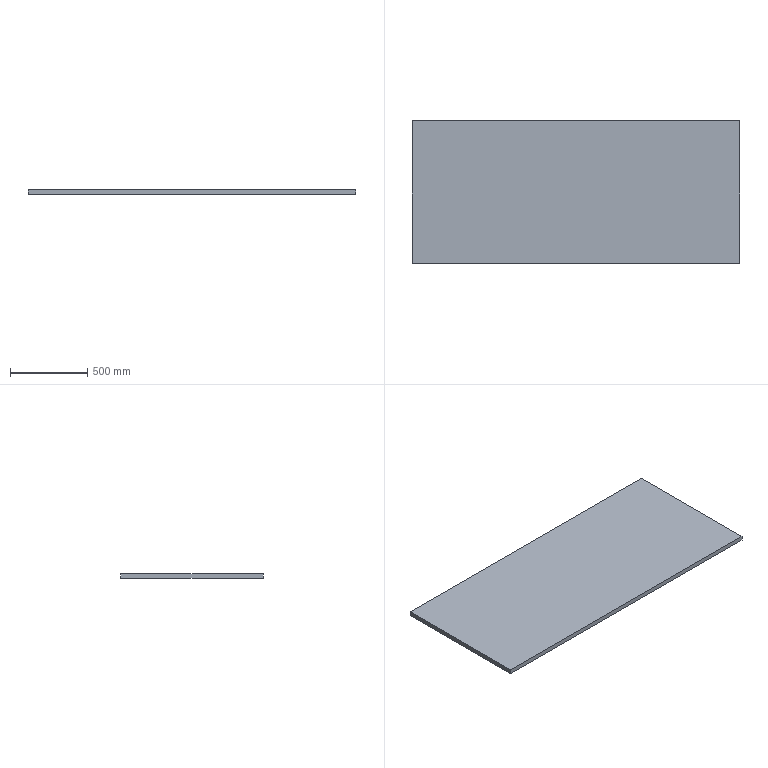Part | SolidWorks | features Extrusion 1 | 1 solid | 6 faces | box 2118 x 922 x 30 mm | volume 58583880 mm3 | plane 6
STEP:
#1=CARTESIAN_POINT('',(0.,922.,0.));
#2=VERTEX_POINT('',#1);
#3=CARTESIAN_POINT('',(0.,0.,0.));
#4=VERTEX_POINT('',#3);
#5=CARTESIAN_POINT('',(0.,0.,0.));
#6=DIRECTION('',(0.,-1.,0.));
#7=VECTOR('',#6,1000.);
#8=LINE('',#5,#7);
#9=EDGE_CURVE('',#2,#4,#8,.T.);
#10=ORIENTED_EDGE('',*,*,#9,.T.);
#11=CARTESIAN_POINT('',(0.,0.,30.));
#12=VERTEX_POINT('',#11);
#13=CARTESIAN_POINT('',(0.,0.,30.));
#14=DIRECTION('',(0.,0.,-1.));
#15=VECTOR('',#14,1000.);
#16=LINE('',#13,#15);
#17=EDGE_CURVE('',#12,#4,#16,.T.);
#18=ORIENTED_EDGE('',*,*,#17,.F.);
#19=CARTESIAN_POINT('',(0.,922.,30.));
#20=VERTEX_POINT('',#19);
#21=CARTESIAN_POINT('',(0.,0.,30.));
#22=DIRECTION('',(0.,-1.,0.));
#23=VECTOR('',#22,1000.);
#24=LINE('',#21,#23);
#25=EDGE_CURVE('',#20,#12,#24,.T.);
#26=ORIENTED_EDGE('',*,*,#25,.F.);
#27=CARTESIAN_POINT('',(0.,922.,30.));
#28=DIRECTION('',(0.,0.,-1.));
#29=VECTOR('',#28,1000.);
#30=LINE('',#27,#29);
#31=EDGE_CURVE('',#20,#2,#30,.T.);
#32=ORIENTED_EDGE('',*,*,#31,.T.);
#33=EDGE_LOOP('',(#10,#18,#26,#32));
#34=FACE_OUTER_BOUND('',#33,.T.);
#35=CARTESIAN_POINT('',(0.,0.,30.));
#36=DIRECTION('',(1.,0.,0.));
#37=DIRECTION('',(0.,0.,-1.));
#38=AXIS2_PLACEMENT_3D('',#35,#36,#37);
#39=PLANE('',#38);
#40=ADVANCED_FACE('',(#34),#39,.F.);
#41=CARTESIAN_POINT('',(2118.,0.,0.));
#42=VERTEX_POINT('',#41);
#43=CARTESIAN_POINT('',(0.,0.,0.));
#44=DIRECTION('',(1.,0.,0.));
#45=VECTOR('',#44,1000.);
#46=LINE('',#43,#45);
#47=EDGE_CURVE('',#4,#42,#46,.T.);
#48=ORIENTED_EDGE('',*,*,#47,.T.);
#49=CARTESIAN_POINT('',(2118.,0.,30.));
#50=VERTEX_POINT('',#49);
#51=CARTESIAN_POINT('',(2118.,0.,30.));
#52=DIRECTION('',(0.,0.,-1.));
#53=VECTOR('',#52,1000.);
#54=LINE('',#51,#53);
#55=EDGE_CURVE('',#50,#42,#54,.T.);
#56=ORIENTED_EDGE('',*,*,#55,.F.);
#57=CARTESIAN_POINT('',(0.,0.,30.));
#58=DIRECTION('',(1.,0.,0.));
#59=VECTOR('',#58,1000.);
#60=LINE('',#57,#59);
#61=EDGE_CURVE('',#12,#50,#60,.T.);
#62=ORIENTED_EDGE('',*,*,#61,.F.);
#63=ORIENTED_EDGE('',*,*,#17,.T.);
#64=EDGE_LOOP('',(#48,#56,#62,#63));
#65=FACE_OUTER_BOUND('',#64,.T.);
#66=CARTESIAN_POINT('',(0.,0.,30.));
#67=DIRECTION('',(0.,1.,0.));
#68=DIRECTION('',(0.,0.,1.));
#69=AXIS2_PLACEMENT_3D('',#66,#67,#68);
#70=PLANE('',#69);
#71=ADVANCED_FACE('',(#65),#70,.F.);
#72=CARTESIAN_POINT('',(2118.,922.,0.));
#73=VERTEX_POINT('',#72);
#74=CARTESIAN_POINT('',(2118.,0.,0.));
#75=DIRECTION('',(0.,1.,0.));
#76=VECTOR('',#75,1000.);
#77=LINE('',#74,#76);
#78=EDGE_CURVE('',#42,#73,#77,.T.);
#79=ORIENTED_EDGE('',*,*,#78,.T.);
#80=CARTESIAN_POINT('',(2118.,922.,30.));
#81=VERTEX_POINT('',#80);
#82=CARTESIAN_POINT('',(2118.,922.,30.));
#83=DIRECTION('',(0.,0.,-1.));
#84=VECTOR('',#83,1000.);
#85=LINE('',#82,#84);
#86=EDGE_CURVE('',#81,#73,#85,.T.);
#87=ORIENTED_EDGE('',*,*,#86,.F.);
#88=CARTESIAN_POINT('',(2118.,0.,30.));
#89=DIRECTION('',(0.,1.,0.));
#90=VECTOR('',#89,1000.);
#91=LINE('',#88,#90);
#92=EDGE_CURVE('',#50,#81,#91,.T.);
#93=ORIENTED_EDGE('',*,*,#92,.F.);
#94=ORIENTED_EDGE('',*,*,#55,.T.);
#95=EDGE_LOOP('',(#79,#87,#93,#94));
#96=FACE_OUTER_BOUND('',#95,.T.);
#97=CARTESIAN_POINT('',(2118.,0.,30.));
#98=DIRECTION('',(-1.,0.,0.));
#99=DIRECTION('',(0.,0.,1.));
#100=AXIS2_PLACEMENT_3D('',#97,#98,#99);
#101=PLANE('',#100);
#102=ADVANCED_FACE('',(#96),#101,.F.);
#103=CARTESIAN_POINT('',(0.,922.,0.));
#104=DIRECTION('',(-1.,0.,0.));
#105=VECTOR('',#104,1000.);
#106=LINE('',#103,#105);
#107=EDGE_CURVE('',#73,#2,#106,.T.);
#108=ORIENTED_EDGE('',*,*,#107,.T.);
#109=ORIENTED_EDGE('',*,*,#31,.F.);
#110=CARTESIAN_POINT('',(0.,922.,30.));
#111=DIRECTION('',(-1.,0.,0.));
#112=VECTOR('',#111,1000.);
#113=LINE('',#110,#112);
#114=EDGE_CURVE('',#81,#20,#113,.T.);
#115=ORIENTED_EDGE('',*,*,#114,.F.);
#116=ORIENTED_EDGE('',*,*,#86,.T.);
#117=EDGE_LOOP('',(#108,#109,#115,#116));
#118=FACE_OUTER_BOUND('',#117,.T.);
#119=CARTESIAN_POINT('',(0.,922.,30.));
#120=DIRECTION('',(0.,-1.,0.));
#121=DIRECTION('',(0.,0.,-1.));
#122=AXIS2_PLACEMENT_3D('',#119,#120,#121);
#123=PLANE('',#122);
#124=ADVANCED_FACE('',(#118),#123,.F.);
#125=ORIENTED_EDGE('',*,*,#25,.T.);
#126=ORIENTED_EDGE('',*,*,#61,.T.);
#127=ORIENTED_EDGE('',*,*,#92,.T.);
#128=ORIENTED_EDGE('',*,*,#114,.T.);
#129=EDGE_LOOP('',(#125,#126,#127,#128));
#130=FACE_OUTER_BOUND('',#129,.T.);
#131=CARTESIAN_POINT('',(0.,0.,30.));
#132=DIRECTION('',(0.,0.,-1.));
#133=DIRECTION('',(-1.,0.,0.));
#134=AXIS2_PLACEMENT_3D('',#131,#132,#133);
#135=PLANE('',#134);
#136=ADVANCED_FACE('',(#130),#135,.F.);
#137=ORIENTED_EDGE('',*,*,#9,.F.);
#138=ORIENTED_EDGE('',*,*,#107,.F.);
#139=ORIENTED_EDGE('',*,*,#78,.F.);
#140=ORIENTED_EDGE('',*,*,#47,.F.);
#141=EDGE_LOOP('',(#137,#138,#139,#140));
#142=FACE_OUTER_BOUND('',#141,.T.);
#143=CARTESIAN_POINT('',(0.,0.,0.));
#144=DIRECTION('',(0.,0.,-1.));
#145=DIRECTION('',(-1.,0.,0.));
#146=AXIS2_PLACEMENT_3D('',#143,#144,#145);
#147=PLANE('',#146);
#148=ADVANCED_FACE('',(#142),#147,.T.);
#149=CLOSED_SHELL('',(#40,#71,#102,#124,#136,#148));
#150=MANIFOLD_SOLID_BREP('',#149);
#151=CARTESIAN_POINT('',(0.,0.,0.));
#152=DIRECTION('',(0.,0.,1.));
#153=DIRECTION('',(1.,0.,0.));
#154=AXIS2_PLACEMENT_3D('',#151,#152,#153);
#155=(LENGTH_UNIT()NAMED_UNIT(*)SI_UNIT(.MILLI.,.METRE.));
#156=UNCERTAINTY_MEASURE_WITH_UNIT(LENGTH_MEASURE(0.00001),#155,'','');
#157=(NAMED_UNIT(*)PLANE_ANGLE_UNIT()SI_UNIT($,.RADIAN.));
#158=(NAMED_UNIT(*)SI_UNIT($,.STERADIAN.)SOLID_ANGLE_UNIT());
#159=(GEOMETRIC_REPRESENTATION_CONTEXT(3)GLOBAL_UNCERTAINTY_ASSIGNED_CONTEXT((#156))GLOBAL_UNIT_ASSIGNED_CONTEXT((#155,#157,#158))REPRESENTATION_CONTEXT('',''));
#160=ADVANCED_BREP_SHAPE_REPRESENTATION('',(#150,#154),#159);